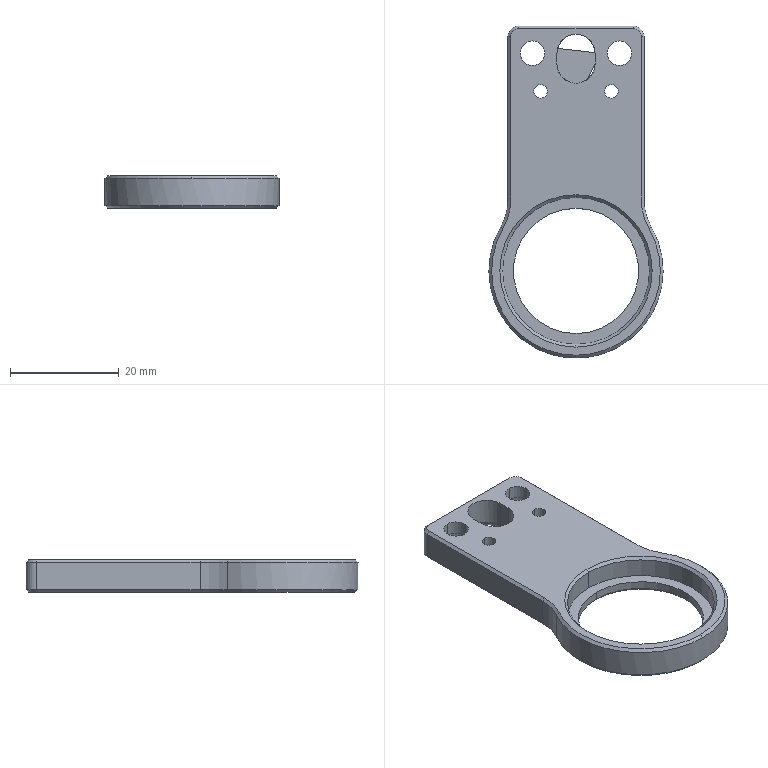NC program | NX | posted with a generic post | part box 32 x 61 x 6 mm
Whole program:
N10 G17 G21 G94 G90
(FLOOR_WALL , TOOL : D80)
N12 T19 M6
N14 G54
N16 G17 G0 G90 X-75.5 Y0. S5000 M3
N18 G43 Z30. H19
N20 Z3.
N22 G94 G1 Z0. F1200.
N24 X-72.5
N26 X72.5
N28 X75.5
N30 Z3.
N32 G0 Z30.
N34 M5
(ZLEVEL_PROFILE , TOOL : D10)
N36 T15 M6
N38 G54
N40 G17 G0 G90 X-35.588 Y-0.401 S9500 M3
N42 G43 Z30. H15
N44 Z1.5
N46 G94 G1 X-35.536 Y1.994 Z1.374 F1000.
N48 X-35.025 Y5.021 Z1.214
N50 X-34.081 Y7.942 Z1.053
N52 X-32.724 Y10.695 Z0.892
N54 X-30.982 Y13.222 Z0.731
N56 X-28.892 Y15.471 Z0.57
N58 X-26.499 Y17.392 Z0.409
N60 X-24.581 Y18.57 Z0.291
N62 X-21.922 Y19.784 Z0.138
N64 X-19.121 Y20.618 Z-0.015
N66 X-16.232 Y21.059 Z-0.168
N68 X-13.31 Y21.096 Z-0.321
N70 X-10.411 Y20.731 Z-0.475
N72 X-7.59 Y19.968 Z-0.628
N74 X-4.901 Y18.824 Z-0.781
N76 X-3.927 Y18.26 Z-0.84
N78 X-3.457 Y17.987 Z-0.868
N80 X-2.014 Y17.6 Z-0.947
N82 X-1.471 Z-0.975
N84 X28.5 F3500.
N86 G2 X35.6 Y10.5 R7.1
N88 G1 Y-10.5
N90 G2 X28.5 Y-17.6 R7.1
N92 G1 X-1.471
N94 G3 X-3.927 Y-18.26 R4.9
N96 G2 X-3.927 Y18.26 R-21.1
N98 G3 X-1.471 Y17.6 R4.9
N100 G1 X28.5 Z-1.124
N102 X29.119 Y17.573 Z-1.127
N104 X29.733 Y17.492 Z-1.13
N106 X30.338 Y17.358 Z-1.133
N108 X30.928 Y17.172 Z-1.136
N110 X31.501 Y16.935 Z-1.139
N112 X32.05 Y16.649 Z-1.142
N114 X32.572 Y16.316 Z-1.145
N116 X33.064 Y15.939 Z-1.148
N118 X33.52 Y15.52 Z-1.151
N120 X33.939 Y15.064 Z-1.154
N122 X34.316 Y14.572 Z-1.157
N124 X34.649 Y14.05 Z-1.16
N126 X34.935 Y13.501 Z-1.163
N128 X35.172 Y12.928 Z-1.166
N130 X35.358 Y12.338 Z-1.17
N132 X35.492 Y11.733 Z-1.173
N134 X35.573 Y11.119 Z-1.176
N136 X35.6 Y10.5 Z-1.179
N138 Y-10.5 Z-1.283
N140 X35.573 Y-11.119 Z-1.286
N142 X35.492 Y-11.733 Z-1.289
N144 X35.358 Y-12.338 Z-1.292
N146 X35.172 Y-12.928 Z-1.295
N148 X34.935 Y-13.501 Z-1.298
N150 X34.649 Y-14.05 Z-1.301
N152 X34.316 Y-14.572 Z-1.304
N154 X33.939 Y-15.064 Z-1.307
N156 X33.52 Y-15.52 Z-1.31
N158 X33.064 Y-15.939 Z-1.313
N160 X32.572 Y-16.316 Z-1.317
N162 X32.05 Y-16.649 Z-1.32
N164 X31.501 Y-16.935 Z-1.323
N166 X30.928 Y-17.172 Z-1.326
N168 X30.338 Y-17.358 Z-1.329
N170 X29.733 Y-17.492 Z-1.332
N172 X29.119 Y-17.573 Z-1.335
N174 X28.5 Y-17.6 Z-1.338
N176 X-1.471 Z-1.486
N178 X-1.899 Y-17.619 Z-1.489
N180 X-2.324 Y-17.675 Z-1.491
N182 X-2.742 Y-17.768 Z-1.493
N184 X-3.151 Y-17.897 Z-1.495
N186 X-3.547 Y-18.061 Z-1.497
N188 X-3.927 Y-18.26 Z-1.499
N190 X-4.869 Y-18.774 Z-1.505
N192 X-5.836 Y-19.239 Z-1.51
N194 X-6.825 Y-19.655 Z-1.515
N196 X-7.835 Y-20.02 Z-1.52
N198 X-8.861 Y-20.333 Z-1.526
N200 X-9.902 Y-20.593 Z-1.531
N202 X-10.956 Y-20.8 Z-1.536
N204 X-12.018 Y-20.953 Z-1.542
N206 X-13.086 Y-21.053 Z-1.547
N208 X-14.159 Y-21.097 Z-1.552
N210 X-15.232 Y-21.087 Z-1.558
N212 X-16.303 Y-21.023 Z-1.563
N214 X-17.37 Y-20.904 Z-1.568
N216 X-18.429 Y-20.731 Z-1.574
N218 X-19.478 Y-20.504 Z-1.579
N220 X-20.514 Y-20.225 Z-1.584
N222 X-21.535 Y-19.893 Z-1.59
N224 X-22.537 Y-19.509 Z-1.595
N226 X-23.519 Y-19.075 Z-1.6
N228 X-24.477 Y-18.592 Z-1.606
N230 X-25.41 Y-18.061 Z-1.611
N232 X-26.314 Y-17.483 Z-1.616
N234 X-27.216 Y-16.838 Z-1.622
N236 X-28.083 Y-16.147 Z-1.627
N238 X-28.912 Y-15.411 Z-1.633
N240 X-29.701 Y-14.633 Z-1.638
N242 X-30.449 Y-13.814 Z-1.644
N244 X-31.153 Y-12.958 Z-1.649
N246 X-31.81 Y-12.065 Z-1.655
N248 X-32.42 Y-11.139 Z-1.66
N250 X-32.98 Y-10.183 Z-1.666
N252 X-33.49 Y-9.198 Z-1.671
N254 X-33.946 Y-8.188 Z-1.677
N256 X-34.35 Y-7.156 Z-1.682
N258 X-34.698 Y-6.103 Z-1.688
N260 X-34.991 Y-5.034 Z-1.693
N262 X-35.227 Y-3.951 Z-1.699
N264 X-35.406 Y-2.857 Z-1.704
N266 X-35.527 Y-1.755 Z-1.71
N268 X-35.59 Y-0.648 Z-1.715
N270 X-35.595 Y0.46 Z-1.721
N272 X-35.542 Y1.568 Z-1.726
N274 X-35.43 Y2.671 Z-1.732
N276 X-35.261 Y3.766 Z-1.737
N278 X-35.035 Y4.851 Z-1.742
N280 X-34.752 Y5.923 Z-1.748
N282 X-34.413 Y6.979 Z-1.753
N284 X-34.018 Y8.015 Z-1.759
N286 X-33.571 Y9.029 Z-1.764
N288 X-33.07 Y10.018 Z-1.77
N290 X-32.518 Y10.98 Z-1.775
N292 X-31.917 Y11.911 Z-1.781
N294 X-31.267 Y12.809 Z-1.786
N296 X-30.571 Y13.672 Z-1.792
N298 X-29.831 Y14.497 Z-1.797
N300 X-29.049 Y15.282 Z-1.803
N302 X-28.226 Y16.025 Z-1.808
N304 X-27.365 Y16.724 Z-1.814
N306 X-26.469 Y17.377 Z-1.819
N308 X-25.54 Y17.981 Z-1.825
N310 X-24.648 Y18.499 Z-1.83
N312 X-23.732 Y18.973 Z-1.835
N314 X-22.794 Y19.402 Z-1.84
N316 X-21.836 Y19.784 Z-1.845
N318 X-20.86 Y20.119 Z-1.85
N320 X-19.869 Y20.405 Z-1.856
N322 X-18.866 Y20.643 Z-1.861
N324 X-17.852 Y20.832 Z-1.866
N326 X-16.83 Y20.971 Z-1.871
N328 X-15.802 Y21.06 Z-1.876
N330 X-14.772 Y21.098 Z-1.881
N332 X-13.74 Y21.086 Z-1.886
N334 X-12.711 Y21.024 Z-1.891
N336 X-11.686 Y20.911 Z-1.896
N338 X-10.667 Y20.749 Z-1.902
N340 X-9.658 Y20.537 Z-1.907
N342 X-8.66 Y20.276 Z-1.912
N344 X-7.676 Y19.966 Z-1.917
N346 X-6.708 Y19.609 Z-1.922
N348 X-5.76 Y19.205 Z-1.927
N350 X-4.832 Y18.754 Z-1.932
N352 X-3.927 Y18.26 Z-1.937
N354 X-3.547 Y18.061 Z-1.939
N356 X-3.151 Y17.897 Z-1.942
N358 X-2.742 Y17.768 Z-1.944
N360 X-2.324 Y17.675 Z-1.946
N362 X-1.899 Y17.619 Z-1.948
N364 X-1.471 Y17.6 Z-1.95
N366 X28.5 Z-2.099
N368 X29.119 Y17.573 Z-2.102
N370 X29.733 Y17.492 Z-2.105
N372 X30.338 Y17.358 Z-2.108
N374 X30.928 Y17.172 Z-2.111
N376 X31.501 Y16.935 Z-2.114
N378 X32.05 Y16.649 Z-2.117
N380 X32.572 Y16.316 Z-2.12
N382 X33.064 Y15.939 Z-2.123
N384 X33.52 Y15.52 Z-2.126
N386 X33.939 Y15.064 Z-2.129
N388 X34.316 Y14.572 Z-2.132
N390 X34.649 Y14.05 Z-2.135
N392 X34.935 Y13.501 Z-2.138
N394 X35.172 Y12.928 Z-2.141
N396 X35.358 Y12.338 Z-2.145
N398 X35.492 Y11.733 Z-2.148
N400 X35.573 Y11.119 Z-2.151
N402 X35.6 Y10.5 Z-2.154
N404 Y-10.5 Z-2.258
N406 X35.573 Y-11.119 Z-2.261
N408 X35.492 Y-11.733 Z-2.264
N410 X35.358 Y-12.338 Z-2.267
N412 X35.172 Y-12.928 Z-2.27
N414 X34.935 Y-13.501 Z-2.273
N416 X34.649 Y-14.05 Z-2.276
N418 X34.316 Y-14.572 Z-2.279
N420 X33.939 Y-15.064 Z-2.282
N422 X33.52 Y-15.52 Z-2.285
N424 X33.064 Y-15.939 Z-2.288
N426 X32.572 Y-16.316 Z-2.292
N428 X32.05 Y-16.649 Z-2.295
N430 X31.501 Y-16.935 Z-2.298
N432 X30.928 Y-17.172 Z-2.301
N434 X30.338 Y-17.358 Z-2.304
N436 X29.733 Y-17.492 Z-2.307
N438 X29.119 Y-17.573 Z-2.31
N440 X28.5 Y-17.6 Z-2.313
N442 X-1.471 Z-2.461
N444 X-1.899 Y-17.619 Z-2.464
N446 X-2.324 Y-17.675 Z-2.466
N448 X-2.742 Y-17.768 Z-2.468
N450 X-3.151 Y-17.897 Z-2.47
N452 X-3.547 Y-18.061 Z-2.472
N454 X-3.927 Y-18.26 Z-2.474
N456 X-4.869 Y-18.774 Z-2.48
N458 X-5.836 Y-19.239 Z-2.485
N460 X-6.825 Y-19.655 Z-2.49
N462 X-7.835 Y-20.02 Z-2.495
N464 X-8.861 Y-20.333 Z-2.501
N466 X-9.902 Y-20.593 Z-2.506
N468 X-10.956 Y-20.8 Z-2.511
N470 X-12.018 Y-20.953 Z-2.517
N472 X-13.086 Y-21.053 Z-2.522
N474 X-14.159 Y-21.097 Z-2.527
N476 X-15.232 Y-21.087 Z-2.533
N478 X-16.303 Y-21.023 Z-2.538
N480 X-17.37 Y-20.904 Z-2.543
N482 X-18.429 Y-20.731 Z-2.549
N484 X-19.478 Y-20.504 Z-2.554
N486 X-20.514 Y-20.225 Z-2.559
N488 X-21.535 Y-19.893 Z-2.565
N490 X-22.537 Y-19.509 Z-2.57
N492 X-23.519 Y-19.075 Z-2.575
N494 X-24.477 Y-18.592 Z-2.581
N496 X-25.41 Y-18.061 Z-2.586
N498 X-26.314 Y-17.483 Z-2.591
N500 X-27.216 Y-16.838 Z-2.597
N502 X-28.083 Y-16.147 Z-2.602
N504 X-28.912 Y-15.411 Z-2.608
N506 X-29.701 Y-14.633 Z-2.613
N508 X-30.449 Y-13.814 Z-2.619
N510 X-31.153 Y-12.958 Z-2.624
N512 X-31.81 Y-12.065 Z-2.63
N514 X-32.42 Y-11.139 Z-2.635
N516 X-32.98 Y-10.183 Z-2.641
N518 X-33.49 Y-9.198 Z-2.646
N520 X-33.946 Y-8.188 Z-2.652
N522 X-34.35 Y-7.156 Z-2.657
N524 X-34.698 Y-6.103 Z-2.663
N526 X-34.991 Y-5.034 Z-2.668
N528 X-35.227 Y-3.951 Z-2.674
N530 X-35.406 Y-2.857 Z-2.679
N532 X-35.527 Y-1.755 Z-2.685
N534 X-35.59 Y-0.648 Z-2.69
N536 X-35.595 Y0.46 Z-2.696
N538 X-35.542 Y1.568 Z-2.701
N540 X-35.43 Y2.671 Z-2.707
N542 X-35.261 Y3.766 Z-2.712
N544 X-35.035 Y4.851 Z-2.717
N546 X-34.752 Y5.923 Z-2.723
N548 X-34.413 Y6.979 Z-2.728
N550 X-34.018 Y8.015 Z-2.734
N552 X-33.571 Y9.029 Z-2.739
N554 X-33.07 Y10.018 Z-2.745
N556 X-32.518 Y10.98 Z-2.75
N558 X-31.917 Y11.911 Z-2.756
N560 X-31.267 Y12.809 Z-2.761
N562 X-30.571 Y13.672 Z-2.767
N564 X-29.831 Y14.497 Z-2.772
N566 X-29.049 Y15.282 Z-2.778
N568 X-28.226 Y16.025 Z-2.783
N570 X-27.365 Y16.724 Z-2.789
N572 X-26.469 Y17.377 Z-2.794
N574 X-25.54 Y17.981 Z-2.8
N576 X-24.648 Y18.499 Z-2.805
N578 X-23.732 Y18.973 Z-2.81
N580 X-22.794 Y19.402 Z-2.815
N582 X-21.836 Y19.784 Z-2.82
N584 X-20.86 Y20.119 Z-2.825
N586 X-19.869 Y20.405 Z-2.831
N588 X-18.866 Y20.643 Z-2.836
N590 X-17.852 Y20.832 Z-2.841
N592 X-16.83 Y20.971 Z-2.846
N594 X-15.802 Y21.06 Z-2.851
N596 X-14.772 Y21.098 Z-2.856
N598 X-13.74 Y21.086 Z-2.861
N600 X-12.711 Y21.024 Z-2.866
N602 X-11.686 Y20.911 Z-2.871
N604 X-10.667 Y20.749 Z-2.877
N606 X-9.658 Y20.537 Z-2.882
N608 X-8.66 Y20.276 Z-2.887
N610 X-7.676 Y19.966 Z-2.892
N612 X-6.708 Y19.609 Z-2.897
N614 X-5.76 Y19.205 Z-2.902
N616 X-4.832 Y18.754 Z-2.907
N618 X-3.927 Y18.26 Z-2.912
N620 X-3.547 Y18.061 Z-2.914
N622 X-3.151 Y17.897 Z-2.917
N624 X-2.742 Y17.768 Z-2.919
N626 X-2.324 Y17.675 Z-2.921
N628 X-1.899 Y17.619 Z-2.923
N630 X-1.471 Y17.6 Z-2.925
N632 X28.5 Z-3.074
N634 X29.119 Y17.573 Z-3.077
N636 X29.733 Y17.492 Z-3.08
N638 X30.338 Y17.358 Z-3.083
N640 X30.928 Y17.172 Z-3.086
N642 X31.501 Y16.935 Z-3.089
N644 X32.05 Y16.649 Z-3.092
N646 X32.572 Y16.316 Z-3.095
N648 X33.064 Y15.939 Z-3.098
N650 X33.52 Y15.52 Z-3.101
N652 X33.939 Y15.064 Z-3.104
N654 X34.316 Y14.572 Z-3.107
N656 X34.649 Y14.05 Z-3.11
N658 X34.935 Y13.501 Z-3.113
N660 X35.172 Y12.928 Z-3.116
N662 X35.358 Y12.338 Z-3.12
N664 X35.492 Y11.733 Z-3.123
N666 X35.573 Y11.119 Z-3.126
N668 X35.6 Y10.5 Z-3.129
N670 Y-10.5 Z-3.233
N672 X35.573 Y-11.119 Z-3.236
N674 X35.492 Y-11.733 Z-3.239
N676 X35.358 Y-12.338 Z-3.242
N678 X35.172 Y-12.928 Z-3.245
N680 X34.935 Y-13.501 Z-3.248
N682 X34.649 Y-14.05 Z-3.251
N684 X34.316 Y-14.572 Z-3.254
N686 X33.939 Y-15.064 Z-3.257
N688 X33.52 Y-15.52 Z-3.26
N690 X33.064 Y-15.939 Z-3.263
N692 X32.572 Y-16.316 Z-3.267
N694 X32.05 Y-16.649 Z-3.27
N696 X31.501 Y-16.935 Z-3.273
N698 X30.928 Y-17.172 Z-3.276
N700 X30.338 Y-17.358 Z-3.279
N702 X29.733 Y-17.492 Z-3.282
N704 X29.119 Y-17.573 Z-3.285
N706 X28.5 Y-17.6 Z-3.288
N708 X-1.471 Z-3.436
N710 X-1.899 Y-17.619 Z-3.439
N712 X-2.324 Y-17.675 Z-3.441
N714 X-2.742 Y-17.768 Z-3.443
N716 X-3.151 Y-17.897 Z-3.445
N718 X-3.547 Y-18.061 Z-3.447
N720 X-3.927 Y-18.26 Z-3.449
N722 X-4.869 Y-18.774 Z-3.455
N724 X-5.836 Y-19.239 Z-3.46
N726 X-6.825 Y-19.655 Z-3.465
N728 X-7.835 Y-20.02 Z-3.47
N730 X-8.861 Y-20.333 Z-3.476
N732 X-9.902 Y-20.593 Z-3.481
N734 X-10.956 Y-20.8 Z-3.486
N736 X-12.018 Y-20.953 Z-3.492
N738 X-13.086 Y-21.053 Z-3.497
N740 X-14.159 Y-21.097 Z-3.502
N742 X-15.232 Y-21.087 Z-3.508
N744 X-16.303 Y-21.023 Z-3.513
N746 X-17.37 Y-20.904 Z-3.518
N748 X-18.429 Y-20.731 Z-3.524
N750 X-19.478 Y-20.504 Z-3.529
N752 X-20.514 Y-20.225 Z-3.534
N754 X-21.535 Y-19.893 Z-3.54
N756 X-22.537 Y-19.509 Z-3.545
N758 X-23.519 Y-19.075 Z-3.55
N760 X-24.477 Y-18.592 Z-3.556
N762 X-25.41 Y-18.061 Z-3.561
N764 X-26.314 Y-17.483 Z-3.566
N766 X-27.216 Y-16.838 Z-3.572
N768 X-28.083 Y-16.147 Z-3.577
N770 X-28.912 Y-15.411 Z-3.583
N772 X-29.701 Y-14.633 Z-3.588
N774 X-30.449 Y-13.814 Z-3.594
N776 X-31.153 Y-12.958 Z-3.599
N778 X-31.81 Y-12.065 Z-3.605
N780 X-32.42 Y-11.139 Z-3.61
N782 X-32.98 Y-10.183 Z-3.616
N784 X-33.49 Y-9.198 Z-3.621
N786 X-33.946 Y-8.188 Z-3.627
N788 X-34.35 Y-7.156 Z-3.632
N790 X-34.698 Y-6.103 Z-3.638
N792 X-34.991 Y-5.034 Z-3.643
N794 X-35.227 Y-3.951 Z-3.649
N796 X-35.406 Y-2.857 Z-3.654
N798 X-35.527 Y-1.755 Z-3.66
N800 X-35.59 Y-0.648 Z-3.665
N802 X-35.595 Y0.46 Z-3.671
N804 X-35.542 Y1.568 Z-3.676
N806 X-35.43 Y2.671 Z-3.682
N808 X-35.261 Y3.766 Z-3.687
N810 X-35.035 Y4.851 Z-3.692
N812 X-34.752 Y5.923 Z-3.698
N814 X-34.413 Y6.979 Z-3.703
N816 X-34.018 Y8.015 Z-3.709
N818 X-33.571 Y9.029 Z-3.714
N820 X-33.07 Y10.018 Z-3.72
N822 X-32.518 Y10.98 Z-3.725
N824 X-31.917 Y11.911 Z-3.731
N826 X-31.267 Y12.809 Z-3.736
N828 X-30.571 Y13.672 Z-3.742
N830 X-29.831 Y14.497 Z-3.747
N832 X-29.049 Y15.282 Z-3.753
N834 X-28.226 Y16.025 Z-3.758
N836 X-27.365 Y16.724 Z-3.764
N838 X-26.469 Y17.377 Z-3.769
N840 X-25.54 Y17.981 Z-3.775
N842 X-24.648 Y18.499 Z-3.78
N844 X-23.732 Y18.973 Z-3.785
N846 X-22.794 Y19.402 Z-3.79
N848 X-21.836 Y19.784 Z-3.795
N850 X-20.86 Y20.119 Z-3.8
N852 X-19.869 Y20.405 Z-3.806
N854 X-18.866 Y20.643 Z-3.811
N856 X-17.852 Y20.832 Z-3.816
N858 X-16.83 Y20.971 Z-3.821
N860 X-15.802 Y21.06 Z-3.826
N862 X-14.772 Y21.098 Z-3.831
N864 X-13.74 Y21.086 Z-3.836
N866 X-12.711 Y21.024 Z-3.841
N868 X-11.686 Y20.911 Z-3.846
N870 X-10.667 Y20.749 Z-3.852
N872 X-9.658 Y20.537 Z-3.857
N874 X-8.66 Y20.276 Z-3.862
N876 X-7.676 Y19.966 Z-3.867
N878 X-6.708 Y19.609 Z-3.872
N880 X-5.76 Y19.205 Z-3.877
N882 X-4.832 Y18.754 Z-3.882
N884 X-3.927 Y18.26 Z-3.887
N886 X-3.547 Y18.061 Z-3.889
N888 X-3.151 Y17.897 Z-3.892
N890 X-2.742 Y17.768 Z-3.894
N892 X-2.324 Y17.675 Z-3.896
N894 X-1.899 Y17.619 Z-3.898
N896 X-1.471 Y17.6 Z-3.9
N898 X28.5 Z-4.007
N900 X29.119 Y17.573 Z-4.009
N902 X29.733 Y17.492 Z-4.011
N904 X30.338 Y17.358 Z-4.013
N906 X30.928 Y17.172 Z-4.015
N908 X31.501 Y16.935 Z-4.018
N910 X32.05 Y16.649 Z-4.02
N912 X32.572 Y16.316 Z-4.022
N914 X33.064 Y15.939 Z-4.024
N916 X33.52 Y15.52 Z-4.026
N918 X33.939 Y15.064 Z-4.029
N920 X34.316 Y14.572 Z-4.031
N922 X34.649 Y14.05 Z-4.033
N924 X34.935 Y13.501 Z-4.035
N926 X35.172 Y12.928 Z-4.037
N928 X35.358 Y12.338 Z-4.04
N930 X35.492 Y11.733 Z-4.042
N932 X35.573 Y11.119 Z-4.044
N934 X35.6 Y10.5 Z-4.046
N936 Y-10.5 Z-4.121
N938 X35.573 Y-11.119 Z-4.123
N940 X35.492 Y-11.733 Z-4.125
N942 X35.358 Y-12.338 Z-4.128
N944 X35.172 Y-12.928 Z-4.13
N946 X34.935 Y-13.501 Z-4.132
N948 X34.649 Y-14.05 Z-4.134
N950 X34.316 Y-14.572 Z-4.136
N952 X33.939 Y-15.064 Z-4.139
N954 X33.52 Y-15.52 Z-4.141
N956 X33.064 Y-15.939 Z-4.143
N958 X32.572 Y-16.316 Z-4.145
N960 X32.05 Y-16.649 Z-4.147
N962 X31.501 Y-16.935 Z-4.15
N964 X30.928 Y-17.172 Z-4.152
N966 X30.338 Y-17.358 Z-4.154
N968 X29.733 Y-17.492 Z-4.156
N970 X29.119 Y-17.573 Z-4.158
N972 X28.5 Y-17.6 Z-4.161
N974 X-1.471 Z-4.267
N976 X-1.899 Y-17.619 Z-4.269
N978 X-2.324 Y-17.675 Z-4.27
N980 X-2.742 Y-17.768 Z-4.272
N982 X-3.151 Y-17.897 Z-4.273
N984 X-3.547 Y-18.061 Z-4.275
N986 X-3.927 Y-18.26 Z-4.276
N988 X-4.869 Y-18.774 Z-4.28
N990 X-5.836 Y-19.239 Z-4.284
N992 X-6.825 Y-19.655 Z-4.288
N994 X-7.835 Y-20.02 Z-4.292
N996 X-8.861 Y-20.333 Z-4.295
N998 X-9.902 Y-20.593 Z-4.299
N1000 X-10.956 Y-20.8 Z-4.303
N1002 X-12.018 Y-20.953 Z-4.307
N1004 X-13.086 Y-21.053 Z-4.311
N1006 X-14.159 Y-21.097 Z-4.315
N1008 X-15.232 Y-21.087 Z-4.318
N1010 X-16.303 Y-21.023 Z-4.322
N1012 X-17.37 Y-20.904 Z-4.326
N1014 X-18.429 Y-20.731 Z-4.33
N1016 X-19.478 Y-20.504 Z-4.334
N1018 X-20.514 Y-20.225 Z-4.337
N1020 X-21.535 Y-19.893 Z-4.341
N1022 X-22.537 Y-19.509 Z-4.345
N1024 X-23.519 Y-19.075 Z-4.349
N1026 X-24.477 Y-18.592 Z-4.353
N1028 X-25.41 Y-18.061 Z-4.357
N1030 X-26.314 Y-17.483 Z-4.36
N1032 X-27.216 Y-16.838 Z-4.364
N1034 X-28.083 Y-16.147 Z-4.368
N1036 X-28.912 Y-15.411 Z-4.372
N1038 X-29.701 Y-14.633 Z-4.376
N1040 X-30.449 Y-13.814 Z-4.38
N1042 X-31.153 Y-12.958 Z-4.384
N1044 X-31.81 Y-12.065 Z-4.388
N1046 X-32.42 Y-11.139 Z-4.392
N1048 X-32.98 Y-10.183 Z-4.396
N1050 X-33.49 Y-9.198 Z-4.4
N1052 X-33.946 Y-8.188 Z-4.404
N1054 X-34.35 Y-7.156 Z-4.408
N1056 X-34.698 Y-6.103 Z-4.412
N1058 X-34.991 Y-5.034 Z-4.416
N1060 X-35.227 Y-3.951 Z-4.419
N1062 X-35.406 Y-2.857 Z-4.423
N1064 X-35.527 Y-1.755 Z-4.427
N1066 X-35.59 Y-0.648 Z-4.431
N1068 X-35.595 Y0.46 Z-4.435
N1070 X-35.542 Y1.568 Z-4.439
N1072 X-35.43 Y2.671 Z-4.443
N1074 X-35.261 Y3.766 Z-4.447
N1076 X-35.035 Y4.851 Z-4.451
N1078 X-34.752 Y5.923 Z-4.455
N1080 X-34.413 Y6.979 Z-4.459
N1082 X-34.018 Y8.015 Z-4.463
N1084 X-33.571 Y9.029 Z-4.467
N1086 X-33.07 Y10.018 Z-4.471
N1088 X-32.518 Y10.98 Z-4.475
N1090 X-31.917 Y11.911 Z-4.479
N1092 X-31.267 Y12.809 Z-4.483
N1094 X-30.571 Y13.672 Z-4.487
N1096 X-29.831 Y14.497 Z-4.49
N1098 X-29.049 Y15.282 Z-4.494
N1100 X-28.226 Y16.025 Z-4.498
N1102 X-27.365 Y16.724 Z-4.502
N1104 X-26.469 Y17.377 Z-4.506
N1106 X-25.54 Y17.981 Z-4.51
N1108 X-24.648 Y18.499 Z-4.514
N1110 X-23.732 Y18.973 Z-4.517
N1112 X-22.794 Y19.402 Z-4.521
N1114 X-21.836 Y19.784 Z-4.525
N1116 X-20.86 Y20.119 Z-4.529
N1118 X-19.869 Y20.405 Z-4.532
N1120 X-18.866 Y20.643 Z-4.536
N1122 X-17.852 Y20.832 Z-4.54
N1124 X-16.83 Y20.971 Z-4.543
N1126 X-15.802 Y21.06 Z-4.547
N1128 X-14.772 Y21.098 Z-4.551
N1130 X-13.74 Y21.086 Z-4.554
N1132 X-12.711 Y21.024 Z-4.558
N1134 X-11.686 Y20.911 Z-4.562
N1136 X-10.667 Y20.749 Z-4.565
N1138 X-9.658 Y20.537 Z-4.569
N1140 X-8.66 Y20.276 Z-4.573
N1142 X-7.676 Y19.966 Z-4.576
N1144 X-6.708 Y19.609 Z-4.58
N1146 X-5.76 Y19.205 Z-4.584
N1148 X-4.832 Y18.754 Z-4.587
N1150 X-3.927 Y18.26 Z-4.591
N1152 X-3.547 Y18.061 Z-4.592
N1154 X-3.151 Y17.897 Z-4.594
N1156 X-2.742 Y17.768 Z-4.595
N1158 X-2.324 Y17.675 Z-4.597
N1160 X-1.899 Y17.619 Z-4.598
N1162 X-1.471 Y17.6 Z-4.6
N1164 X28.5 Z-4.707
N1166 X29.119 Y17.573 Z-4.709
N1168 X29.733 Y17.492 Z-4.711
N1170 X30.338 Y17.358 Z-4.713
N1172 X30.928 Y17.172 Z-4.715
N1174 X31.501 Y16.935 Z-4.718
N1176 X32.05 Y16.649 Z-4.72
N1178 X32.572 Y16.316 Z-4.722
N1180 X33.064 Y15.939 Z-4.724
N1182 X33.52 Y15.52 Z-4.726
N1184 X33.939 Y15.064 Z-4.729
N1186 X34.316 Y14.572 Z-4.731
N1188 X34.649 Y14.05 Z-4.733
N1190 X34.935 Y13.501 Z-4.735
N1192 X35.172 Y12.928 Z-4.737
N1194 X35.358 Y12.338 Z-4.74
N1196 X35.492 Y11.733 Z-4.742
N1198 X35.573 Y11.119 Z-4.744
N1200 X35.6 Y10.5 Z-4.746
N1202 Y-10.5 Z-4.821
N1204 X35.573 Y-11.119 Z-4.823
N1206 X35.492 Y-11.733 Z-4.825
N1208 X35.358 Y-12.338 Z-4.828
N1210 X35.172 Y-12.928 Z-4.83
N1212 X34.935 Y-13.501 Z-4.832
N1214 X34.649 Y-14.05 Z-4.834
N1216 X34.316 Y-14.572 Z-4.836
N1218 X33.939 Y-15.064 Z-4.839
N1220 X33.52 Y-15.52 Z-4.841
N1222 X33.064 Y-15.939 Z-4.843
N1224 X32.572 Y-16.316 Z-4.845
N1226 X32.05 Y-16.649 Z-4.847
N1228 X31.501 Y-16.935 Z-4.85
N1230 X30.928 Y-17.172 Z-4.852
N1232 X30.338 Y-17.358 Z-4.854
N1234 X29.733 Y-17.492 Z-4.856
N1236 X29.119 Y-17.573 Z-4.858
N1238 X28.5 Y-17.6 Z-4.861
N1240 X-1.471 Z-4.967
N1242 X-1.899 Y-17.619 Z-4.969
N1244 X-2.324 Y-17.675 Z-4.97
N1246 X-2.742 Y-17.768 Z-4.972
N1248 X-3.151 Y-17.897 Z-4.973
N1250 X-3.547 Y-18.061 Z-4.975
N1252 X-3.927 Y-18.26 Z-4.976
N1254 X-4.869 Y-18.774 Z-4.98
N1256 X-5.836 Y-19.239 Z-4.984
N1258 X-6.825 Y-19.655 Z-4.988
N1260 X-7.835 Y-20.02 Z-4.992
N1262 X-8.861 Y-20.333 Z-4.995
N1264 X-9.902 Y-20.593 Z-4.999
N1266 X-10.956 Y-20.8 Z-5.003
N1268 X-12.018 Y-20.953 Z-5.007
N1270 X-13.086 Y-21.053 Z-5.011
N1272 X-14.159 Y-21.097 Z-5.015
N1274 X-15.232 Y-21.087 Z-5.018
N1276 X-16.303 Y-21.023 Z-5.022
N1278 X-17.37 Y-20.904 Z-5.026
N1280 X-18.429 Y-20.731 Z-5.03
N1282 X-19.478 Y-20.504 Z-5.034
N1284 X-20.514 Y-20.225 Z-5.037
N1286 X-21.535 Y-19.893 Z-5.041
N1288 X-22.537 Y-19.509 Z-5.045
N1290 X-23.519 Y-19.075 Z-5.049
N1292 X-24.477 Y-18.592 Z-5.053
N1294 X-25.41 Y-18.061 Z-5.057
N1296 X-26.314 Y-17.483 Z-5.06
N1298 X-27.216 Y-16.838 Z-5.064
N1300 X-28.083 Y-16.147 Z-5.068
N1302 X-28.912 Y-15.411 Z-5.072
N1304 X-29.701 Y-14.633 Z-5.076
N1306 X-30.449 Y-13.814 Z-5.08
N1308 X-31.153 Y-12.958 Z-5.084
N1310 X-31.81 Y-12.065 Z-5.088
N1312 X-32.42 Y-11.139 Z-5.092
N1314 X-32.98 Y-10.183 Z-5.096
N1316 X-33.49 Y-9.198 Z-5.1
N1318 X-33.946 Y-8.188 Z-5.104
N1320 X-34.35 Y-7.156 Z-5.108
N1322 X-34.698 Y-6.103 Z-5.112
N1324 X-34.991 Y-5.034 Z-5.116
N1326 X-35.227 Y-3.951 Z-5.119
N1328 X-35.406 Y-2.857 Z-5.123
N1330 X-35.527 Y-1.755 Z-5.127
N1332 X-35.59 Y-0.648 Z-5.131
N1334 X-35.595 Y0.46 Z-5.135
N1336 X-35.542 Y1.568 Z-5.139
N1338 X-35.43 Y2.671 Z-5.143
N1340 X-35.261 Y3.766 Z-5.147
N1342 X-35.035 Y4.851 Z-5.151
N1344 X-34.752 Y5.923 Z-5.155
N1346 X-34.413 Y6.979 Z-5.159
N1348 X-34.018 Y8.015 Z-5.163
N1350 X-33.571 Y9.029 Z-5.167
N1352 X-33.07 Y10.018 Z-5.171
N1354 X-32.518 Y10.98 Z-5.175
N1356 X-31.917 Y11.911 Z-5.179
N1358 X-31.267 Y12.809 Z-5.183
N1360 X-30.571 Y13.672 Z-5.187
N1362 X-29.831 Y14.497 Z-5.19
N1364 X-29.049 Y15.282 Z-5.194
N1366 X-28.226 Y16.025 Z-5.198
N1368 X-27.365 Y16.724 Z-5.202
N1370 X-26.469 Y17.377 Z-5.206
N1372 X-25.54 Y17.981 Z-5.21
N1374 X-24.648 Y18.499 Z-5.214
N1376 X-23.732 Y18.973 Z-5.217
N1378 X-22.794 Y19.402 Z-5.221
N1380 X-21.836 Y19.784 Z-5.225
N1382 X-20.86 Y20.119 Z-5.229
N1384 X-19.869 Y20.405 Z-5.232
N1386 X-18.866 Y20.643 Z-5.236
N1388 X-17.852 Y20.832 Z-5.24
N1390 X-16.83 Y20.971 Z-5.243
N1392 X-15.802 Y21.06 Z-5.247
N1394 X-14.772 Y21.098 Z-5.251
N1396 X-13.74 Y21.086 Z-5.254
N1398 X-12.711 Y21.024 Z-5.258
N1400 X-11.686 Y20.911 Z-5.262
N1402 X-10.667 Y20.749 Z-5.265
N1404 X-9.658 Y20.537 Z-5.269
N1406 X-8.66 Y20.276 Z-5.273
N1408 X-7.676 Y19.966 Z-5.276
N1410 X-6.708 Y19.609 Z-5.28
N1412 X-5.76 Y19.205 Z-5.284
N1414 X-4.832 Y18.754 Z-5.287
N1416 X-3.927 Y18.26 Z-5.291
N1418 X-3.547 Y18.061 Z-5.292
N1420 X-3.151 Y17.897 Z-5.294
N1422 X-2.742 Y17.768 Z-5.295
N1424 X-2.324 Y17.675 Z-5.297
N1426 X-1.899 Y17.619 Z-5.298
N1428 X-1.471 Y17.6 Z-5.3
N1430 X28.5 Z-5.407
N1432 X29.119 Y17.573 Z-5.409
N1434 X29.733 Y17.492 Z-5.411
N1436 X30.338 Y17.358 Z-5.413
N1438 X30.928 Y17.172 Z-5.415
N1440 X31.501 Y16.935 Z-5.418
N1442 X32.05 Y16.649 Z-5.42
N1444 X32.572 Y16.316 Z-5.422
N1446 X33.064 Y15.939 Z-5.424
N1448 X33.52 Y15.52 Z-5.426
N1450 X33.939 Y15.064 Z-5.429
N1452 X34.316 Y14.572 Z-5.431
N1454 X34.649 Y14.05 Z-5.433
N1456 X34.935 Y13.501 Z-5.435
N1458 X35.172 Y12.928 Z-5.437
N1460 X35.358 Y12.338 Z-5.44
N1462 X35.492 Y11.733 Z-5.442
N1464 X35.573 Y11.119 Z-5.444
N1466 X35.6 Y10.5 Z-5.446
N1468 Y-10.5 Z-5.521
N1470 X35.573 Y-11.119 Z-5.523
N1472 X35.492 Y-11.733 Z-5.525
N1474 X35.358 Y-12.338 Z-5.528
N1476 X35.172 Y-12.928 Z-5.53
N1478 X34.935 Y-13.501 Z-5.532
N1480 X34.649 Y-14.05 Z-5.534
N1482 X34.316 Y-14.572 Z-5.536
N1484 X33.939 Y-15.064 Z-5.539
N1486 X33.52 Y-15.52 Z-5.541
N1488 X33.064 Y-15.939 Z-5.543
N1490 X32.572 Y-16.316 Z-5.545
N1492 X32.05 Y-16.649 Z-5.547
N1494 X31.501 Y-16.935 Z-5.55
N1496 X30.928 Y-17.172 Z-5.552
N1498 X30.338 Y-17.358 Z-5.554
N1500 X29.733 Y-17.492 Z-5.556
N1502 X29.119 Y-17.573 Z-5.558
N1504 X28.5 Y-17.6 Z-5.561
N1506 X-1.471 Z-5.667
N1508 X-1.899 Y-17.619 Z-5.669
N1510 X-2.324 Y-17.675 Z-5.67
N1512 X-2.742 Y-17.768 Z-5.672
N1514 X-3.151 Y-17.897 Z-5.673
N1516 X-3.547 Y-18.061 Z-5.675
N1518 X-3.927 Y-18.26 Z-5.676
N1520 X-4.869 Y-18.774 Z-5.68
N1522 X-5.836 Y-19.239 Z-5.684
N1524 X-6.825 Y-19.655 Z-5.688
N1526 X-7.835 Y-20.02 Z-5.692
N1528 X-8.861 Y-20.333 Z-5.695
N1530 X-9.902 Y-20.593 Z-5.699
N1532 X-10.956 Y-20.8 Z-5.703
N1534 X-12.018 Y-20.953 Z-5.707
N1536 X-13.086 Y-21.053 Z-5.711
N1538 X-14.159 Y-21.097 Z-5.715
N1540 X-15.232 Y-21.087 Z-5.718
N1542 X-16.303 Y-21.023 Z-5.722
N1544 X-17.37 Y-20.904 Z-5.726
N1546 X-18.429 Y-20.731 Z-5.73
N1548 X-19.478 Y-20.504 Z-5.734
N1550 X-20.514 Y-20.225 Z-5.737
N1552 X-21.535 Y-19.893 Z-5.741
N1554 X-22.537 Y-19.509 Z-5.745
N1556 X-23.519 Y-19.075 Z-5.749
N1558 X-24.477 Y-18.592 Z-5.753
N1560 X-25.41 Y-18.061 Z-5.757
N1562 X-26.314 Y-17.483 Z-5.76
N1564 X-27.216 Y-16.838 Z-5.764
N1566 X-28.083 Y-16.147 Z-5.768
N1568 X-28.912 Y-15.411 Z-5.772
N1570 X-29.701 Y-14.633 Z-5.776
N1572 X-30.449 Y-13.814 Z-5.78
N1574 X-31.153 Y-12.958 Z-5.784
N1576 X-31.81 Y-12.065 Z-5.788
N1578 X-32.42 Y-11.139 Z-5.792
N1580 X-32.98 Y-10.183 Z-5.796
N1582 X-33.49 Y-9.198 Z-5.8
N1584 X-33.946 Y-8.188 Z-5.804
N1586 X-34.35 Y-7.156 Z-5.808
N1588 X-34.698 Y-6.103 Z-5.812
N1590 X-34.991 Y-5.034 Z-5.816
N1592 X-35.227 Y-3.951 Z-5.819
N1594 X-35.406 Y-2.857 Z-5.823
N1596 X-35.527 Y-1.755 Z-5.827
N1598 X-35.59 Y-0.648 Z-5.831
N1600 X-35.595 Y0.46 Z-5.835
N1602 X-35.542 Y1.568 Z-5.839
N1604 X-35.43 Y2.671 Z-5.843
N1606 X-35.261 Y3.766 Z-5.847
N1608 X-35.035 Y4.851 Z-5.851
N1610 X-34.752 Y5.923 Z-5.855
N1612 X-34.413 Y6.979 Z-5.859
N1614 X-34.018 Y8.015 Z-5.863
N1616 X-33.571 Y9.029 Z-5.867
N1618 X-33.07 Y10.018 Z-5.871
N1620 X-32.518 Y10.98 Z-5.875
N1622 X-31.917 Y11.911 Z-5.879
N1624 X-31.267 Y12.809 Z-5.883
N1626 X-30.571 Y13.672 Z-5.887
N1628 X-29.831 Y14.497 Z-5.89
N1630 X-29.049 Y15.282 Z-5.894
N1632 X-28.226 Y16.025 Z-5.898
N1634 X-27.365 Y16.724 Z-5.902
N1636 X-26.469 Y17.377 Z-5.906
N1638 X-25.54 Y17.981 Z-5.91
N1640 X-24.648 Y18.499 Z-5.914
N1642 X-23.732 Y18.973 Z-5.917
N1644 X-22.794 Y19.402 Z-5.921
N1646 X-21.836 Y19.784 Z-5.925
N1648 X-20.86 Y20.119 Z-5.929
N1650 X-19.869 Y20.405 Z-5.932
N1652 X-18.866 Y20.643 Z-5.936
N1654 X-17.852 Y20.832 Z-5.94
N1656 X-16.83 Y20.971 Z-5.943
N1658 X-15.802 Y21.06 Z-5.947
N1660 X-14.772 Y21.098 Z-5.951
N1662 X-13.74 Y21.086 Z-5.954
N1664 X-12.711 Y21.024 Z-5.958
N1666 X-11.686 Y20.911 Z-5.962
N1668 X-10.667 Y20.749 Z-5.965
N1670 X-9.658 Y20.537 Z-5.969
N1672 X-8.66 Y20.276 Z-5.973
N1674 X-7.676 Y19.966 Z-5.976
N1676 X-6.708 Y19.609 Z-5.98
N1678 X-5.76 Y19.205 Z-5.984
N1680 X-4.832 Y18.754 Z-5.987
N1682 X-3.927 Y18.26 Z-5.991
N1684 X-3.547 Y18.061 Z-5.992
N1686 X-3.151 Y17.897 Z-5.994
N1688 X-2.742 Y17.768 Z-5.995
N1690 X-2.324 Y17.675 Z-5.997
N1692 X-1.899 Y17.619 Z-5.998
N1694 X-1.471 Y17.6 Z-6.
N1696 X28.5
N1698 G2 X35.6 Y10.5 R7.1
N1700 G1 Y-10.5
N1702 G2 X28.5 Y-17.6 R7.1
N1704 G1 X-1.471
N1706 G3 X-3.927 Y-18.26 R4.9
N1708 G2 X-3.927 Y18.26 R-21.1
N1710 G3 X-1.471 Y17.6 R4.9
N1712 G1 Z-4.5
N1714 G0 Z30.
(HOLE_MILLING_COPY , TOOL : D10)
N1716 X-14.5 Y0.
N1718 Z0.
N1720 G3 X-15.75 Y-1.25 R1.25 F1000.
N1722 X-14.5 Y-2.5 R1.25
N1724 X-14.5 Y-2.5 Z-1. I0. J2.5 F2500.
N1726 X-14.5 Y-2.5 Z-2. I0. J2.5
N1728 X-14.5 Y-2.5 Z-3. I0. J2.5
N1730 X-14.5 Y-2.5 Z-4. I0. J2.5
N1732 X-11.823 Y0.17 R2.677
N1734 X-14.484 Y2.999 R2.826
N1736 X-17.745 Y0.095 R3.086
N1738 X-14.537 Y-3.498 R3.404
N1740 X-10.756 Y-0.118 R3.585
N1742 X-14.437 Y3.997 R3.904
N1744 X-18.743 Y0.146 R4.085
N1746 X-14.594 Y-4.496 R4.403
N1748 X-9.759 Y-0.18 R4.585
N1750 X-14.369 Y4.994 R4.903
N1752 X-19.739 Y0.219 R5.084
N1754 X-14.673 Y-5.492 R5.402
N1756 X-8.763 Y-0.264 R5.583
N1758 X-14.28 Y5.99 R5.901
N1760 X-20.735 Y0.313 R6.083
N1762 X-14.772 Y-6.488 R6.401
N1764 X-7.768 Y-0.368 R6.582
N1766 X-14.171 Y6.985 R6.9
N1768 X-21.728 Y0.428 R7.081
N1770 X-14.892 Y-7.481 R7.399
N1772 X-6.776 Y-0.493 R7.581
N1774 X-14.04 Y7.978 R7.899
N1776 X-22.817 Y0.334 R8.16
N1778 X-15.033 Y-8.473 R8.322
N1780 X-6.027 Y-0.533 R8.49
N1782 X-15.033 Y-8.473 R-8.49
N1784 X-10.53 Y-4.503 R4.245
N1786 X-14.5 Y0. R4.245
N1788 G0 Z30.
(HOLE_MILLING_COPY_COPY , TOOL : D10)
N1790 Z-3.5
N1792 G3 X-15.75 Y-1.25 R1.25 F1000.
N1794 X-14.5 Y-2.5 R1.25
N1796 X-14.5 Y-2.5 Z-4.5 I0. J2.5 F2500.
N1798 X-14.5 Y-2.5 Z-5.5 I0. J2.5
N1800 X-14.5 Y2.5 Z-6. I0. J2.5
N1802 X-17.177 Y-0.177 R2.677
N1804 X-14.5 Y-3. R2.827
N1806 X-11.253 Y-0.069 R3.087
N1808 X-14.5 Y3.5 R3.405
N1810 X-18.247 Y0.069 R3.587
N1812 X-14.5 Y-4. R3.906
N1814 X-10.253 Y-0.069 R4.088
N1816 X-14.5 Y4.5 R4.406
N1818 X-19.248 Y0.069 R4.588
N1820 X-14.5 Y-5. R4.907
N1822 X-9.252 Y-0.069 R5.088
N1824 X-14.5 Y5.5 R5.407
N1826 X-20.248 Y0.069 R5.589
N1828 X-14.5 Y-6. R5.907
N1830 X-8.167 Y0.167 R6.169
N1832 X-14.5 Y6.5 R6.333
N1834 X-21. Y0. R6.5
N1836 X-14.5 Y6.5 R-6.5
N1838 X-17.75 Y3.25 R3.25
N1840 X-14.5 Y0. R3.25
N1842 G0 Z30.
N1844 M5
(ZLEVEL_PROFILE_COPY , TOOL : D10JING)
N1846 T14 M6
N1848 G54
N1850 G17 G0 G90 X-20.67 Y-2.043 S9500 M3
N1852 G43 Z30. H14
N1854 Z-4.5
N1856 G94 G1 X-20.605 Y-2.317 Z-4.515 F1000.
N1858 X-19.793 Y-3.825 Z-4.605
N1860 X-18.616 Y-5.069 Z-4.694
N1862 X-17.156 Y-5.965 Z-4.784
N1864 X-15.513 Y-6.451 Z-4.874
N1866 X-13.801 Y-6.492 Z-4.964
N1868 X-12.136 Y-6.087 Z-5.053
N1870 X-11.019 Y-5.525 Z-5.119
N1872 X-9.864 Y-4.599 Z-5.197
N1874 X-8.947 Y-3.436 Z-5.274
N1876 X-8.316 Y-2.096 Z-5.352
N1878 X-8.002 Y-0.649 Z-5.429
N1880 X-7.998 Y0.601 Z-5.495
N1882 X-8.292 Y2.024 Z-5.571
N1884 X-8.893 Y3.347 Z-5.647
N1886 X-9.772 Y4.504 Z-5.723
N1888 X-10.885 Y5.438 Z-5.799
N1890 X-11.988 Y6.027 Z-5.865
N1892 X-12.914 Y6.334 Z-5.916
N1894 X-13.875 Y6.5 Z-5.967
N1896 X-14.5 Z-6.
N1898 G3 X-21. Y0. R6.5 F1500.
N1900 X-14.5 Y6.5 R-6.5
N1902 G1 Z-4.5
N1904 G0 Z30.
N1906 X-28.212 Y15.89
N1908 Z-4.5
N1910 G1 X-26.429 Y17.32 Z-4.62 F1000.
N1912 X-24.514 Y18.493 Z-4.737
N1914 X-21.87 Y19.696 Z-4.89
N1916 X-19.085 Y20.524 Z-5.042
N1918 X-16.213 Y20.96 Z-5.194
N1920 X-13.308 Y20.996 Z-5.346
N1922 X-10.426 Y20.632 Z-5.499
N1924 X-7.622 Y19.873 Z-5.651
N1926 X-4.948 Y18.736 Z-5.803
N1928 X-3.977 Y18.173 Z-5.862
N1930 X-3.502 Y17.898 Z-5.891
N1932 X-2.02 Y17.5 Z-5.971
N1934 X-1.471 Z-6.
N1936 X28.5 F1500.
N1938 G2 X35.5 Y10.5 R7.
N1940 G1 Y-10.5
N1942 G2 X28.5 Y-17.5 R7.
N1944 G1 X-1.471
N1946 G3 X-3.977 Y-18.173 R5.
N1948 G2 X-3.977 Y18.173 R-21.
N1950 G3 X-1.471 Y17.5 R5.
N1952 G1 Z-4.5
N1954 G0 Z30.
N1956 M5
(SPOT_DRILLING , TOOL : D6A45)
N1958 T01 M6
N1960 G54
N1962 G17 G0 G90 X18.5 Y6.5 S9500 M3
N1964 G43 Z30. H1
N1966 G94 G82 G98 Z-1. F250. P200 R3.
N1968 Y-6.5
N1970 X25.5 Y8.
N1972 Y-8.
N1974 G80
N1976 G0 X25.5 Y-8. Z30.
N1978 M5
(DRILLING_COPY_COPY_COPY , TOOL : 2.5ZT)
N1980 T02 M6
N1982 G54
N1984 G17 G0 G90 X18.5 Y6.5 S2500 M3
N1986 G43 Z30. H2
N1988 G94 G83 G98 Z-8.251 F100. Q2. R3.
N1990 Y-6.5
N1992 G80
N1994 G0 X18.5 Y-6.5 Z30.
N1996 M5
(DRILLING , TOOL : 4.5ZT)
N1998 T08 M6
N2000 G54
N2002 G17 G0 G90 X25.5 Y8. S2500 M3
N2004 G43 Z30. H8
N2006 G94 G83 G98 Z-5.352 F200. Q2. R3.
N2008 Y-8.
N2010 G80
N2012 G0 X25.5 Y-8. Z30.
N2014 M5
(PLANAR_PROFILE , TOOL : D6A45)
N2016 T01 M6
N2018 G54
N2020 G17 G0 G90 X18.455 Y-6.8 S9500 M3
N2022 G43 Z30. H1
N2024 Z0.5
N2026 G94 G1 X18.637 Z0.451 F500.
N2028 X18.8 Y-6.637 Z0.389
N2030 Y-6.363 Z0.316
N2032 X18.637 Y-6.2 Z0.254
N2034 X18.363 Z0.181
N2036 X18.2 Y-6.363 Z0.119
N2038 Y-6.637 Z0.045
N2040 X18.363 Y-6.8 Z-0.016
N2042 X18.637 Z-0.09
N2044 X18.8 Y-6.637 Z-0.152
N2046 Y-6.363 Z-0.225
N2048 X18.637 Y-6.2 Z-0.287
N2050 X18.363 Z-0.361
N2052 X18.2 Y-6.363 Z-0.422
N2054 Y-6.637 Z-0.496
N2056 X18.363 Y-6.8 Z-0.557
N2058 X18.637 Z-0.631
N2060 X18.8 Y-6.637 Z-0.693
N2062 Y-6.363 Z-0.766
N2064 X18.637 Y-6.2 Z-0.828
N2066 X18.363 Z-0.902
N2068 X18.2 Y-6.363 Z-0.963
N2070 Y-6.5 Z-1.
N2072 G3 X18.5 Y-6.8 R0.3 F1500.
N2074 X18.2 Y-6.5 R-0.3
N2076 X18.35 Y-6.76 R0.3
N2078 G1 Z0.5
N2080 G0 Z30.
N2082 X25.234 Y-7.862
N2084 Z0.5
N2086 G1 Z-1. F500.
N2088 X24.5 Y-7.48
N2090 G3 X24.2 Y-8. R0.6
N2092 X25.5 Y-9.3 R1.3 F1500.
N2094 X24.2 Y-8. R-1.3
N2096 X24.5 Y-8.52 R0.6
N2098 G1 X25.234 Y-8.138
N2100 Z0.5
N2102 G0 Z30.
N2104 X25.849 Y1.51
N2106 Z0.5
N2108 G1 Z-1. F500.
N2110 X26.02 Y2.25
N2112 G3 X25.5 Y2.55 R0.6
N2114 G1 X23.5 F1500.
N2116 G3 X20.95 Y0. R2.55
N2118 X23.5 Y-2.55 R2.55
N2120 G1 X25.5
N2122 G3 X28.05 Y0. R2.55
N2124 X25.5 Y2.55 R2.55
N2126 X24.98 Y2.25 R0.6
N2128 G1 X24.576 Y1.55
N2130 Z0.5
N2132 G0 Z30.
N2134 X25.766 Y7.862
N2136 Z0.5
N2138 G1 Z-1. F500.
N2140 X26.5 Y7.48
N2142 G3 X26.8 Y8. R0.6
N2144 X25.5 Y9.3 R1.3 F1500.
N2146 X26.8 Y8. R-1.3
N2148 X26.5 Y8.52 R0.6
N2150 G1 X25.766 Y8.138
N2152 Z0.5
N2154 G0 Z30.
N2156 X18.455 Y6.2
N2158 Z0.5
N2160 G1 X18.637 Z0.451 F500.
N2162 X18.8 Y6.363 Z0.389
N2164 Y6.637 Z0.316
N2166 X18.637 Y6.8 Z0.254
N2168 X18.363 Z0.181
N2170 X18.2 Y6.637 Z0.119
N2172 Y6.363 Z0.045
N2174 X18.363 Y6.2 Z-0.016
N2176 X18.637 Z-0.09
N2178 X18.8 Y6.363 Z-0.152
N2180 Y6.637 Z-0.225
N2182 X18.637 Y6.8 Z-0.287
N2184 X18.363 Z-0.361
N2186 X18.2 Y6.637 Z-0.422
N2188 Y6.363 Z-0.496
N2190 X18.363 Y6.2 Z-0.557
N2192 X18.637 Z-0.631
N2194 X18.8 Y6.363 Z-0.693
N2196 Y6.637 Z-0.766
N2198 X18.637 Y6.8 Z-0.828
N2200 X18.363 Z-0.902
N2202 X18.2 Y6.637 Z-0.963
N2204 Y6.5 Z-1.
N2206 G3 X18.5 Y6.2 R0.3 F1500.
N2208 X18.2 Y6.5 R-0.3
N2210 X18.35 Y6.24 R0.3
N2212 G1 Z0.5
N2214 G0 Z30.
N2216 X-4.903 Y-14.669
N2218 Z0.5
N2220 G1 Z-1. F500.
N2222 X-5.657 Y-14.235
N2224 G3 X-6.257 Y-14.236 R0.6
N2226 G2 X-6.257 Y14.236 R-16.45 F1500.
N2228 G3 X-1.471 Y12.95 R9.55
N2230 G1 X28.5
N2232 G2 X30.95 Y10.5 R2.45
N2234 G1 Y-10.5
N2236 G2 X28.5 Y-12.95 R2.45
N2238 G1 X-1.471
N2240 G3 X-6.257 Y-14.236 R9.55
N2242 X-6.556 Y-14.756 R0.6
N2244 G1 X-6.555 Y-15.536
N2246 Z0.5
N2248 G0 Z30.
N2250 X-2.487 Y-0.945
N2252 Z0.5
N2254 G1 Z-1. F500.
N2256 X-1.75 Y-0.52
N2258 G3 X-1.45 Y0. R0.6
N2260 X-14.5 Y13.05 R13.05 F1500.
N2262 X-1.45 Y0. R-13.05
N2264 X-1.75 Y0.52 R0.6
N2266 G1 X-2.487 Y0.945
N2268 Z0.5
N2270 G0 Z30.
N2272 M5
(刀补 , TOOL : D10)
N2274 T15 M6
N2276 G54
N2278 G17 G0 G90 X-14.5 Y0. S9500 M3
N2280 G43 Z30. H15
N2282 Z0.
N2284 G41 G94 G1 X-17.142 Y-4.813 F1000. D15
N2286 G3 X-14.5 Y-8.5 R2.79
N2288 X-14.5 Y-8.5 Z-2. I0. J8.5 F1500.
N2290 X-14.5 Y-8.5 Z-4. I0. J8.5
N2292 X-6. Y0. R8.5
N2294 X-14.5 Y-8.5 R-8.5
N2296 X-11.858 Y-4.813 R2.79
N2298 G40
N2300 G1 X-14.5 Y0.
N2302 G0 Z30.
N2304 M5
N2306 M2